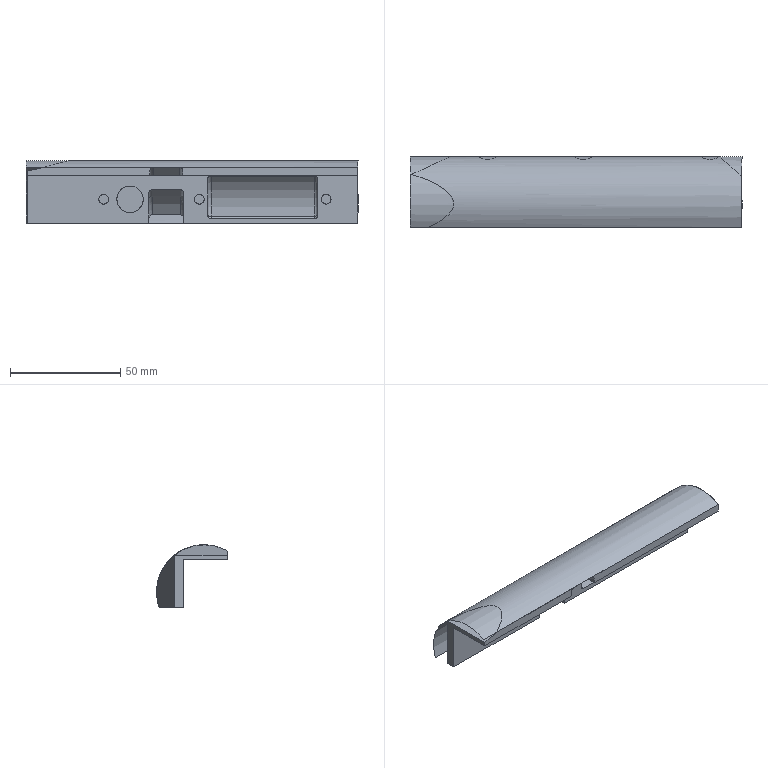NC program | Mastercam | posted with a generic post
Lines 25152 to 25225 of 52802:
(10 FEM |TOOL - 10|DIA. OFF. - 10|LEN. - 10|TOOL DIA. - 10.)
N872 T10 M6
N874 G0 G54 G90 X81. Y-10.413 C0. B0. S6000 M3
N876 G43 H10 Z25.
N878 Z-18.993
N880 G1 Z-19.993 F600.
N882 X75. F1000.
N884 X-75.
N886 X-81.
N888 Y-3.913
N890 X-75.
N892 X75.
N894 X81.
N896 Y2.587
N898 X75.
N900 X-75.
N902 X-81.
N904 X81. Y2.597
N906 X75.
N908 X-75.
N910 X-81.
N912 G0 Z25.
N914 X-28.8 Y-3.698
N916 Z-24.493
N918 G1 Z-25.493 F600.
N920 Y-3.998 F300.
N922 G3 X-28.5 Y-4.298 I.3
N924 X-27.5 Y-3.298 J1.
N926 X-28.5 Y-2.298 I-1.
N928 X-29.5 Y-3.298 J-1.
N930 X-28.5 Y-4.298 I1.
N932 X-28.021 Y-4.176 J1.
N934 X-27.864 Y-3.912 I-.143 J.264
N936 X-27.901 Y-3.768 I-.3
N938 G1 X-28.045 Y-3.505
N940 G0 Z25.
N942 X-75.3 Y19.773
N944 Z1.
N946 G1 Z-16.5 F600.
N948 Y19.473 F1000.
N950 G3 X-75. Y19.173 I.3
N952 G1 X75.
N954 G2 X80. Y14.173 J-5.
N956 G1 Y-14.173
N958 G2 X75. Y-19.173 I-5.
N960 G1 X-75.
N962 G2 X-80. Y-14.173 J5.
N964 G1 Y14.173
N966 G2 X-75. Y19.173 I5.
N968 G1 X-74.5
N970 G3 X-74.2 Y19.473 J.3
N972 G1 Y19.773
N974 X-75.3
N976 Z-33. F600.
N978 Y19.473 F1000.
N980 G3 X-75. Y19.173 I.3
N982 G1 X75.
N984 G2 X80. Y14.173 J-5.
N986 G1 Y-14.173
N988 G2 X75. Y-19.173 I-5.
N990 G1 X-75.
N992 G2 X-80. Y-14.173 J5.
N994 G1 Y14.173
N996 G2 X-75. Y19.173 I5.
N998 G1 X-74.5
N1000 G3 X-74.2 Y19.473 J.3
N1002 G1 Y19.773
N1004 G0 Z25.
N1006 M5
N1008 G0 G28 G91 Z0.
N1010 G28
N1012 M01
N1014 G0 G17 G40 G80 G90 G94 G98
N1016 G0 G28 G91 Z0.